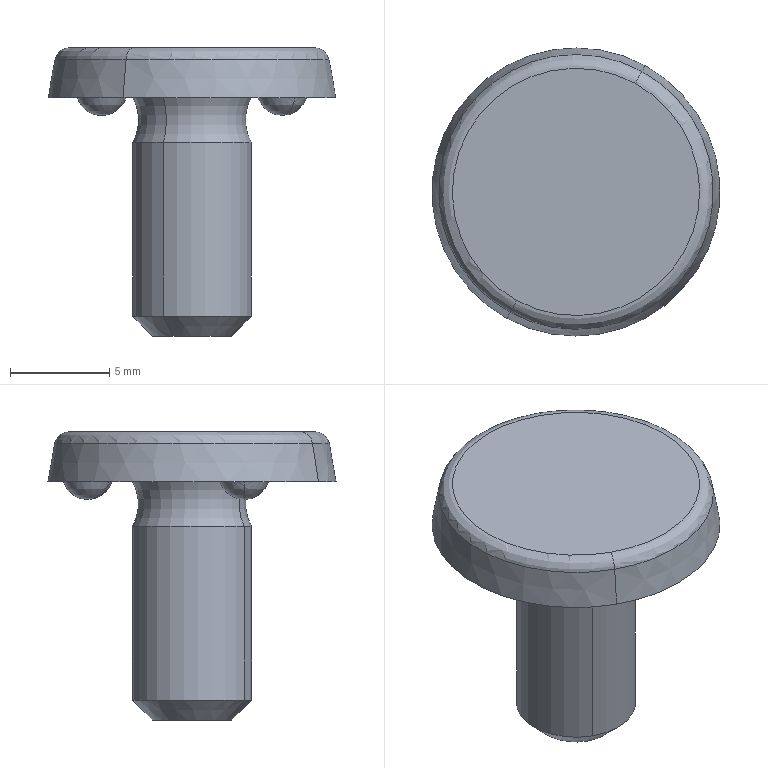Part | STEP file | Q1980612 | 1 solid | 19 faces | box 14.5 x 14.5 x 14.5 mm | volume 715.577 mm3 | sphere 6 | cone 4 | torus 4 | plane 3 | cylinder 2 | commonest cylinder face diameters 6 x2
STEP:
#1=CARTESIAN_POINT('',(4.547,-2.625,-0.9));
#2=VERTEX_POINT('',#1);
#3=CARTESIAN_POINT('',(5.19,-3.681,0.));
#4=VERTEX_POINT('',#3);
#5=CARTESIAN_POINT('',(4.547,-2.625,0.4));
#6=DIRECTION('',(0.854,0.5203,0.));
#7=AXIS2_PLACEMENT_3D('',#5,#6,$);
#8=CIRCLE('',#7,1.3);
#9=EDGE_CURVE('',#2,#4,#8,.F.);
#10=ORIENTED_EDGE('',*,*,#9,.F.);
#11=CARTESIAN_POINT('',(3.903,-1.569,0.));
#12=VERTEX_POINT('',#11);
#13=CARTESIAN_POINT('',(4.547,-2.625,0.4));
#14=DIRECTION('',(-0.854,-0.5203,0.));
#15=AXIS2_PLACEMENT_3D('',#13,#14,$);
#16=CIRCLE('',#15,1.3);
#17=EDGE_CURVE('',#2,#12,#16,.F.);
#18=ORIENTED_EDGE('',*,*,#17,.T.);
#19=CARTESIAN_POINT('',(5.19,-3.681,0.));
#20=CARTESIAN_POINT('',(5.46,-3.517,0.));
#21=CARTESIAN_POINT('',(5.678,-3.266,0.));
#22=CARTESIAN_POINT('',(5.805,-2.951,0.));
#23=CARTESIAN_POINT('',(5.832,-2.453,0.));
#24=CARTESIAN_POINT('',(5.639,-2.013,0.));
#25=CARTESIAN_POINT('',(5.551,-1.877,0.));
#26=CARTESIAN_POINT('',(5.238,-1.532,0.));
#27=CARTESIAN_POINT('',(4.79,-1.354,0.));
#28=CARTESIAN_POINT('',(4.468,-1.333,0.));
#29=CARTESIAN_POINT('',(4.161,-1.411,0.));
#30=CARTESIAN_POINT('',(3.903,-1.569,0.));
#31=B_SPLINE_CURVE_WITH_KNOTS('',5,(#19,#20,#21,#22,#23,#24,#25,#26,#27,#28,#29,#30),.UNSPECIFIED.,.F.,.U.,(6,3,3,6),(0.,2.294,3.444,5.637),.UNSPECIFIED.);
#32=EDGE_CURVE('',#4,#12,#31,.T.);
#33=ORIENTED_EDGE('',*,*,#32,.F.);
#34=EDGE_LOOP('',(#10,#18,#33));
#35=FACE_OUTER_BOUND('',#34,.T.);
#36=CARTESIAN_POINT('',(4.547,-2.625,0.4));
#37=DIRECTION('',(0.,0.,-1.));
#38=DIRECTION('',(0.5203,-0.854,0.));
#39=AXIS2_PLACEMENT_3D('',#36,#37,#38);
#40=SPHERICAL_SURFACE('',#39,1.3);
#41=ADVANCED_FACE('',(#35),#40,.T.);
#42=ORIENTED_EDGE('',*,*,#17,.F.);
#43=ORIENTED_EDGE('',*,*,#9,.T.);
#44=CARTESIAN_POINT('',(5.19,-3.681,0.));
#45=CARTESIAN_POINT('',(4.92,-3.846,0.));
#46=CARTESIAN_POINT('',(4.598,-3.924,0.));
#47=CARTESIAN_POINT('',(4.259,-3.893,0.));
#48=CARTESIAN_POINT('',(3.804,-3.689,0.));
#49=CARTESIAN_POINT('',(3.502,-3.315,0.));
#50=CARTESIAN_POINT('',(3.422,-3.175,0.));
#51=CARTESIAN_POINT('',(3.258,-2.738,0.));
#52=CARTESIAN_POINT('',(3.305,-2.258,0.));
#53=CARTESIAN_POINT('',(3.435,-1.962,0.));
#54=CARTESIAN_POINT('',(3.645,-1.726,0.));
#55=CARTESIAN_POINT('',(3.903,-1.569,0.));
#56=B_SPLINE_CURVE_WITH_KNOTS('',5,(#44,#45,#46,#47,#48,#49,#50,#51,#52,#53,#54,#55),.UNSPECIFIED.,.F.,.U.,(6,3,3,6),(0.,2.294,3.444,5.637),.UNSPECIFIED.);
#57=EDGE_CURVE('',#4,#12,#56,.T.);
#58=ORIENTED_EDGE('',*,*,#57,.T.);
#59=EDGE_LOOP('',(#42,#43,#58));
#60=FACE_OUTER_BOUND('',#59,.T.);
#61=ADVANCED_FACE('',(#60),#40,.T.);
#62=CARTESIAN_POINT('',(-3.476,-6.362,0.));
#63=VERTEX_POINT('',#62);
#64=CARTESIAN_POINT('',(3.476,6.362,0.));
#65=VERTEX_POINT('',#64);
#66=CARTESIAN_POINT('',(0.,0.,0.));
#67=DIRECTION('',(0.,0.,-1.));
#68=AXIS2_PLACEMENT_3D('',#66,#67,$);
#69=CIRCLE('',#68,7.25);
#70=EDGE_CURVE('',#63,#65,#69,.T.);
#71=ORIENTED_EDGE('',*,*,#70,.T.);
#72=CARTESIAN_POINT('',(0.,0.,0.));
#73=DIRECTION('',(0.,0.,-1.));
#74=AXIS2_PLACEMENT_3D('',#72,#73,$);
#75=CIRCLE('',#74,7.25);
#76=EDGE_CURVE('',#65,#63,#75,.T.);
#77=ORIENTED_EDGE('',*,*,#76,.T.);
#78=EDGE_LOOP('',(#71,#77));
#79=FACE_OUTER_BOUND('',#78,.T.);
#80=CARTESIAN_POINT('',(1.438,2.633,0.));
#81=VERTEX_POINT('',#80);
#82=CARTESIAN_POINT('',(-1.438,-2.633,0.));
#83=VERTEX_POINT('',#82);
#84=CARTESIAN_POINT('',(0.,0.,0.));
#85=DIRECTION('',(0.,0.,-1.));
#86=AXIS2_PLACEMENT_3D('',#84,#85,$);
#87=CIRCLE('',#86,3.);
#88=EDGE_CURVE('',#81,#83,#87,.T.);
#89=ORIENTED_EDGE('',*,*,#88,.F.);
#90=CARTESIAN_POINT('',(0.,0.,0.));
#91=DIRECTION('',(0.,0.,-1.));
#92=AXIS2_PLACEMENT_3D('',#90,#91,$);
#93=CIRCLE('',#92,3.);
#94=EDGE_CURVE('',#83,#81,#93,.T.);
#95=ORIENTED_EDGE('',*,*,#94,.F.);
#96=EDGE_LOOP('',(#89,#95));
#97=FACE_BOUND('',#96,.T.);
#98=CARTESIAN_POINT('',(-5.783,-2.654,0.));
#99=VERTEX_POINT('',#98);
#100=CARTESIAN_POINT('',(-3.31,-2.596,0.));
#101=VERTEX_POINT('',#100);
#102=CARTESIAN_POINT('',(-5.783,-2.654,0.));
#103=CARTESIAN_POINT('',(-5.787,-2.497,0.));
#104=CARTESIAN_POINT('',(-5.766,-2.338,0.));
#105=CARTESIAN_POINT('',(-5.719,-2.185,0.));
#106=CARTESIAN_POINT('',(-5.578,-1.897,0.));
#107=CARTESIAN_POINT('',(-5.355,-1.668,0.));
#108=CARTESIAN_POINT('',(-5.225,-1.572,0.));
#109=CARTESIAN_POINT('',(-4.939,-1.425,0.));
#110=CARTESIAN_POINT('',(-4.622,-1.375,0.));
#111=CARTESIAN_POINT('',(-4.46,-1.376,0.));
#112=CARTESIAN_POINT('',(-4.144,-1.429,0.));
#113=CARTESIAN_POINT('',(-3.859,-1.578,0.));
#114=CARTESIAN_POINT('',(-3.73,-1.675,0.));
#115=CARTESIAN_POINT('',(-3.519,-1.896,0.));
#116=CARTESIAN_POINT('',(-3.383,-2.17,0.));
#117=CARTESIAN_POINT('',(-3.338,-2.309,0.));
#118=CARTESIAN_POINT('',(-3.313,-2.452,0.));
#119=CARTESIAN_POINT('',(-3.31,-2.596,0.));
#120=B_SPLINE_CURVE_WITH_KNOTS('',5,(#102,#103,#104,#105,#106,#107,#108,#109,#110,#111,#112,#113,#114,#115,#116,#117,#118,#119),.UNSPECIFIED.,.F.,.U.,(6,3,3,3,3,6),(0.,1.143,2.294,3.444,4.595,5.637),.UNSPECIFIED.);
#121=EDGE_CURVE('',#99,#101,#120,.T.);
#122=ORIENTED_EDGE('',*,*,#121,.F.);
#123=CARTESIAN_POINT('',(-5.783,-2.654,0.));
#124=CARTESIAN_POINT('',(-5.78,-2.812,0.));
#125=CARTESIAN_POINT('',(-5.751,-2.969,0.));
#126=CARTESIAN_POINT('',(-5.697,-3.12,0.));
#127=CARTESIAN_POINT('',(-5.543,-3.4,0.));
#128=CARTESIAN_POINT('',(-5.309,-3.619,0.));
#129=CARTESIAN_POINT('',(-5.174,-3.709,0.));
#130=CARTESIAN_POINT('',(-4.882,-3.842,0.));
#131=CARTESIAN_POINT('',(-4.563,-3.877,0.));
#132=CARTESIAN_POINT('',(-4.402,-3.869,0.));
#133=CARTESIAN_POINT('',(-4.088,-3.801,0.));
#134=CARTESIAN_POINT('',(-3.811,-3.638,0.));
#135=CARTESIAN_POINT('',(-3.686,-3.535,0.));
#136=CARTESIAN_POINT('',(-3.485,-3.304,0.));
#137=CARTESIAN_POINT('',(-3.363,-3.024,0.));
#138=CARTESIAN_POINT('',(-3.324,-2.884,0.));
#139=CARTESIAN_POINT('',(-3.307,-2.74,0.));
#140=CARTESIAN_POINT('',(-3.31,-2.596,0.));
#141=B_SPLINE_CURVE_WITH_KNOTS('',5,(#123,#124,#125,#126,#127,#128,#129,#130,#131,#132,#133,#134,#135,#136,#137,#138,#139,#140),.UNSPECIFIED.,.F.,.U.,(6,3,3,3,3,6),(0.,1.143,2.294,3.444,4.595,5.637),.UNSPECIFIED.);
#142=EDGE_CURVE('',#99,#101,#141,.T.);
#143=ORIENTED_EDGE('',*,*,#142,.T.);
#144=EDGE_LOOP('',(#122,#143));
#145=FACE_BOUND('',#144,.T.);
#146=CARTESIAN_POINT('',(0.593,6.336,0.));
#147=VERTEX_POINT('',#146);
#148=CARTESIAN_POINT('',(-0.593,4.164,0.));
#149=VERTEX_POINT('',#148);
#150=CARTESIAN_POINT('',(0.593,6.336,0.));
#151=CARTESIAN_POINT('',(0.7313,6.26,0.));
#152=CARTESIAN_POINT('',(0.8576,6.162,0.));
#153=CARTESIAN_POINT('',(0.9672,6.045,0.));
#154=CARTESIAN_POINT('',(1.146,5.779,0.));
#155=CARTESIAN_POINT('',(1.233,5.471,0.));
#156=CARTESIAN_POINT('',(1.251,5.311,0.));
#157=CARTESIAN_POINT('',(1.235,4.99,0.));
#158=CARTESIAN_POINT('',(1.12,4.69,0.));
#159=CARTESIAN_POINT('',(1.039,4.551,0.));
#160=CARTESIAN_POINT('',(0.8345,4.303,0.));
#161=CARTESIAN_POINT('',(0.5629,4.131,0.));
#162=CARTESIAN_POINT('',(0.4143,4.068,0.));
#163=CARTESIAN_POINT('',(0.1169,3.995,0.));
#164=CARTESIAN_POINT('',(-0.188,4.015,0.));
#165=CARTESIAN_POINT('',(-0.3307,4.045,0.));
#166=CARTESIAN_POINT('',(-0.4669,4.096,0.));
#167=CARTESIAN_POINT('',(-0.593,4.164,0.));
#168=B_SPLINE_CURVE_WITH_KNOTS('',5,(#150,#151,#152,#153,#154,#155,#156,#157,#158,#159,#160,#161,#162,#163,#164,#165,#166,#167),.UNSPECIFIED.,.F.,.U.,(6,3,3,3,3,6),(0.,1.143,2.294,3.444,4.595,5.637),.UNSPECIFIED.);
#169=EDGE_CURVE('',#147,#149,#168,.T.);
#170=ORIENTED_EDGE('',*,*,#169,.F.);
#171=CARTESIAN_POINT('',(0.593,6.336,0.));
#172=CARTESIAN_POINT('',(0.4547,6.411,0.));
#173=CARTESIAN_POINT('',(0.3043,6.465,0.));
#174=CARTESIAN_POINT('',(0.1466,6.494,0.));
#175=CARTESIAN_POINT('',(-0.1735,6.5,0.));
#176=CARTESIAN_POINT('',(-0.4798,6.407,0.));
#177=CARTESIAN_POINT('',(-0.6246,6.335,0.));
#178=CARTESIAN_POINT('',(-0.8862,6.149,0.));
#179=CARTESIAN_POINT('',(-1.076,5.89,0.));
#180=CARTESIAN_POINT('',(-1.15,5.746,0.));
#181=CARTESIAN_POINT('',(-1.248,5.44,0.));
#182=CARTESIAN_POINT('',(-1.245,5.119,0.));
#183=CARTESIAN_POINT('',(-1.218,4.96,0.));
#184=CARTESIAN_POINT('',(-1.119,4.67,0.));
#185=CARTESIAN_POINT('',(-0.9379,4.424,0.));
#186=CARTESIAN_POINT('',(-0.8353,4.321,0.));
#187=CARTESIAN_POINT('',(-0.7192,4.233,0.));
#188=CARTESIAN_POINT('',(-0.593,4.164,0.));
#189=B_SPLINE_CURVE_WITH_KNOTS('',5,(#171,#172,#173,#174,#175,#176,#177,#178,#179,#180,#181,#182,#183,#184,#185,#186,#187,#188),.UNSPECIFIED.,.F.,.U.,(6,3,3,3,3,6),(0.,1.143,2.294,3.444,4.595,5.637),.UNSPECIFIED.);
#190=EDGE_CURVE('',#147,#149,#189,.T.);
#191=ORIENTED_EDGE('',*,*,#190,.T.);
#192=EDGE_LOOP('',(#170,#191));
#193=FACE_BOUND('',#192,.T.);
#194=ORIENTED_EDGE('',*,*,#57,.F.);
#195=ORIENTED_EDGE('',*,*,#32,.T.);
#196=EDGE_LOOP('',(#194,#195));
#197=FACE_BOUND('',#196,.T.);
#198=CARTESIAN_POINT('',(0.,3.,0.));
#199=DIRECTION('',(0.,0.,-1.));
#200=DIRECTION('',(1.,0.,0.));
#201=AXIS2_PLACEMENT_3D('',#198,#199,#200);
#202=PLANE('',#201);
#203=ADVANCED_FACE('',(#79,#97,#145,#193,#197),#202,.T.);
#204=ORIENTED_EDGE('',*,*,#70,.F.);
#205=CARTESIAN_POINT('',(-3.313,-6.065,1.922));
#206=VERTEX_POINT('',#205);
#207=CARTESIAN_POINT('',(-3.395,-6.214,0.9608));
#208=DIRECTION('',(-0.08325,-0.1524,-0.9848));
#209=VECTOR('',#208,1.);
#210=LINE('',#207,#209);
#211=EDGE_CURVE('',#63,#206,#210,.F.);
#212=ORIENTED_EDGE('',*,*,#211,.T.);
#213=CARTESIAN_POINT('',(3.313,6.065,1.922));
#214=VERTEX_POINT('',#213);
#215=CARTESIAN_POINT('',(0.,0.,1.922));
#216=DIRECTION('',(0.,0.,-1.));
#217=AXIS2_PLACEMENT_3D('',#215,#216,$);
#218=CIRCLE('',#217,6.911);
#219=EDGE_CURVE('',#206,#214,#218,.T.);
#220=ORIENTED_EDGE('',*,*,#219,.T.);
#221=CARTESIAN_POINT('',(3.395,6.214,0.9608));
#222=DIRECTION('',(0.08325,0.1524,-0.9848));
#223=VECTOR('',#222,1.);
#224=LINE('',#221,#223);
#225=EDGE_CURVE('',#65,#214,#224,.F.);
#226=ORIENTED_EDGE('',*,*,#225,.F.);
#227=EDGE_LOOP('',(#204,#212,#220,#226));
#228=FACE_OUTER_BOUND('',#227,.T.);
#229=CARTESIAN_POINT('',(0.,0.,1.922));
#230=DIRECTION('',(0.,0.,-1.));
#231=DIRECTION('',(0.4794,0.8776,0.));
#232=AXIS2_PLACEMENT_3D('',#229,#230,#231);
#233=CONICAL_SURFACE('',#232,6.911,0.1745);
#234=ADVANCED_FACE('',(#228),#233,.T.);
#235=ORIENTED_EDGE('',*,*,#76,.F.);
#236=ORIENTED_EDGE('',*,*,#225,.T.);
#237=CARTESIAN_POINT('',(0.,0.,1.922));
#238=DIRECTION('',(0.,0.,-1.));
#239=AXIS2_PLACEMENT_3D('',#237,#238,$);
#240=CIRCLE('',#239,6.911);
#241=EDGE_CURVE('',#214,#206,#240,.T.);
#242=ORIENTED_EDGE('',*,*,#241,.T.);
#243=ORIENTED_EDGE('',*,*,#211,.F.);
#244=EDGE_LOOP('',(#235,#236,#242,#243));
#245=FACE_OUTER_BOUND('',#244,.T.);
#246=ADVANCED_FACE('',(#245),#233,.T.);
#247=CARTESIAN_POINT('',(1.438,2.633,-2.25));
#248=VERTEX_POINT('',#247);
#249=CARTESIAN_POINT('',(-1.438,-2.633,-2.25));
#250=VERTEX_POINT('',#249);
#251=CARTESIAN_POINT('',(0.,0.,-2.25));
#252=DIRECTION('',(0.,0.,-1.));
#253=AXIS2_PLACEMENT_3D('',#251,#252,$);
#254=CIRCLE('',#253,3.);
#255=EDGE_CURVE('',#248,#250,#254,.T.);
#256=ORIENTED_EDGE('',*,*,#255,.F.);
#257=CARTESIAN_POINT('',(2.372,4.343,-1.125));
#258=DIRECTION('',(-0.8776,0.4794,0.));
#259=AXIS2_PLACEMENT_3D('',#257,#258,$);
#260=CIRCLE('',#259,2.25);
#261=EDGE_CURVE('',#248,#81,#260,.T.);
#262=ORIENTED_EDGE('',*,*,#261,.T.);
#263=ORIENTED_EDGE('',*,*,#88,.T.);
#264=CARTESIAN_POINT('',(-2.372,-4.343,-1.125));
#265=DIRECTION('',(0.8776,-0.4794,0.));
#266=AXIS2_PLACEMENT_3D('',#264,#265,$);
#267=CIRCLE('',#266,2.25);
#268=EDGE_CURVE('',#250,#83,#267,.T.);
#269=ORIENTED_EDGE('',*,*,#268,.F.);
#270=EDGE_LOOP('',(#256,#262,#263,#269));
#271=FACE_OUTER_BOUND('',#270,.T.);
#272=CARTESIAN_POINT('',(0.,0.,-1.125));
#273=DIRECTION('',(0.,0.,-1.));
#274=DIRECTION('',(0.4794,0.8776,0.));
#275=AXIS2_PLACEMENT_3D('',#272,#273,#274);
#276=TOROIDAL_SURFACE('',#275,4.949,2.25);
#277=ADVANCED_FACE('',(#271),#276,.F.);
#278=CARTESIAN_POINT('',(0.,0.,-2.25));
#279=DIRECTION('',(0.,0.,-1.));
#280=AXIS2_PLACEMENT_3D('',#278,#279,$);
#281=CIRCLE('',#280,3.);
#282=EDGE_CURVE('',#250,#248,#281,.T.);
#283=ORIENTED_EDGE('',*,*,#282,.F.);
#284=ORIENTED_EDGE('',*,*,#268,.T.);
#285=ORIENTED_EDGE('',*,*,#94,.T.);
#286=ORIENTED_EDGE('',*,*,#261,.F.);
#287=EDGE_LOOP('',(#283,#284,#285,#286));
#288=FACE_OUTER_BOUND('',#287,.T.);
#289=ADVANCED_FACE('',(#288),#276,.F.);
#290=CARTESIAN_POINT('',(-4.547,-2.625,-0.9));
#291=VERTEX_POINT('',#290);
#292=CARTESIAN_POINT('',(-4.547,-2.625,0.4));
#293=DIRECTION('',(-0.0236,0.9997,0.));
#294=AXIS2_PLACEMENT_3D('',#292,#293,$);
#295=CIRCLE('',#294,1.3);
#296=EDGE_CURVE('',#291,#101,#295,.F.);
#297=ORIENTED_EDGE('',*,*,#296,.F.);
#298=CARTESIAN_POINT('',(-4.547,-2.625,0.4));
#299=DIRECTION('',(0.0236,-0.9997,0.));
#300=AXIS2_PLACEMENT_3D('',#298,#299,$);
#301=CIRCLE('',#300,1.3);
#302=EDGE_CURVE('',#291,#99,#301,.F.);
#303=ORIENTED_EDGE('',*,*,#302,.T.);
#304=ORIENTED_EDGE('',*,*,#121,.T.);
#305=EDGE_LOOP('',(#297,#303,#304));
#306=FACE_OUTER_BOUND('',#305,.T.);
#307=CARTESIAN_POINT('',(-4.547,-2.625,0.4));
#308=DIRECTION('',(0.,0.,-1.));
#309=DIRECTION('',(-0.9997,-0.0236,0.));
#310=AXIS2_PLACEMENT_3D('',#307,#308,#309);
#311=SPHERICAL_SURFACE('',#310,1.3);
#312=ADVANCED_FACE('',(#306),#311,.T.);
#313=ORIENTED_EDGE('',*,*,#302,.F.);
#314=ORIENTED_EDGE('',*,*,#296,.T.);
#315=ORIENTED_EDGE('',*,*,#142,.F.);
#316=EDGE_LOOP('',(#313,#314,#315));
#317=FACE_OUTER_BOUND('',#316,.T.);
#318=ADVANCED_FACE('',(#317),#311,.T.);
#319=CARTESIAN_POINT('',(0.,5.25,-0.9));
#320=VERTEX_POINT('',#319);
#321=CARTESIAN_POINT('',(0.,5.25,0.4));
#322=DIRECTION('',(0.8776,-0.4794,0.));
#323=AXIS2_PLACEMENT_3D('',#321,#322,$);
#324=CIRCLE('',#323,1.3);
#325=EDGE_CURVE('',#320,#149,#324,.F.);
#326=ORIENTED_EDGE('',*,*,#325,.F.);
#327=CARTESIAN_POINT('',(0.,5.25,0.4));
#328=DIRECTION('',(-0.8776,0.4794,0.));
#329=AXIS2_PLACEMENT_3D('',#327,#328,$);
#330=CIRCLE('',#329,1.3);
#331=EDGE_CURVE('',#320,#147,#330,.F.);
#332=ORIENTED_EDGE('',*,*,#331,.T.);
#333=ORIENTED_EDGE('',*,*,#169,.T.);
#334=EDGE_LOOP('',(#326,#332,#333));
#335=FACE_OUTER_BOUND('',#334,.T.);
#336=CARTESIAN_POINT('',(0.,5.25,0.4));
#337=DIRECTION('',(0.,0.,-1.));
#338=DIRECTION('',(0.4794,0.8776,0.));
#339=AXIS2_PLACEMENT_3D('',#336,#337,#338);
#340=SPHERICAL_SURFACE('',#339,1.3);
#341=ADVANCED_FACE('',(#335),#340,.T.);
#342=ORIENTED_EDGE('',*,*,#331,.F.);
#343=ORIENTED_EDGE('',*,*,#325,.T.);
#344=ORIENTED_EDGE('',*,*,#190,.F.);
#345=EDGE_LOOP('',(#342,#343,#344));
#346=FACE_OUTER_BOUND('',#345,.T.);
#347=ADVANCED_FACE('',(#346),#340,.T.);
#348=ORIENTED_EDGE('',*,*,#219,.F.);
#349=CARTESIAN_POINT('',(-2.983,-5.46,2.5));
#350=VERTEX_POINT('',#349);
#351=CARTESIAN_POINT('',(-2.983,-5.46,1.8));
#352=DIRECTION('',(0.8776,-0.4794,0.));
#353=AXIS2_PLACEMENT_3D('',#351,#352,$);
#354=CIRCLE('',#353,0.7);
#355=EDGE_CURVE('',#206,#350,#354,.F.);
#356=ORIENTED_EDGE('',*,*,#355,.T.);
#357=CARTESIAN_POINT('',(2.983,5.46,2.5));
#358=VERTEX_POINT('',#357);
#359=CARTESIAN_POINT('',(0.,0.,2.5));
#360=DIRECTION('',(0.,0.,-1.));
#361=AXIS2_PLACEMENT_3D('',#359,#360,$);
#362=CIRCLE('',#361,6.222);
#363=EDGE_CURVE('',#350,#358,#362,.T.);
#364=ORIENTED_EDGE('',*,*,#363,.T.);
#365=CARTESIAN_POINT('',(2.983,5.46,1.8));
#366=DIRECTION('',(-0.8776,0.4794,0.));
#367=AXIS2_PLACEMENT_3D('',#365,#366,$);
#368=CIRCLE('',#367,0.7);
#369=EDGE_CURVE('',#214,#358,#368,.F.);
#370=ORIENTED_EDGE('',*,*,#369,.F.);
#371=EDGE_LOOP('',(#348,#356,#364,#370));
#372=FACE_OUTER_BOUND('',#371,.T.);
#373=CARTESIAN_POINT('',(0.,0.,1.8));
#374=DIRECTION('',(0.,0.,-1.));
#375=DIRECTION('',(0.4794,0.8776,0.));
#376=AXIS2_PLACEMENT_3D('',#373,#374,#375);
#377=TOROIDAL_SURFACE('',#376,6.222,0.7);
#378=ADVANCED_FACE('',(#372),#377,.T.);
#379=ORIENTED_EDGE('',*,*,#241,.F.);
#380=ORIENTED_EDGE('',*,*,#369,.T.);
#381=CARTESIAN_POINT('',(0.,0.,2.5));
#382=DIRECTION('',(0.,0.,-1.));
#383=AXIS2_PLACEMENT_3D('',#381,#382,$);
#384=CIRCLE('',#383,6.222);
#385=EDGE_CURVE('',#358,#350,#384,.T.);
#386=ORIENTED_EDGE('',*,*,#385,.T.);
#387=ORIENTED_EDGE('',*,*,#355,.F.);
#388=EDGE_LOOP('',(#379,#380,#386,#387));
#389=FACE_OUTER_BOUND('',#388,.T.);
#390=ADVANCED_FACE('',(#389),#377,.T.);
#391=CARTESIAN_POINT('',(1.438,2.633,-11.));
#392=VERTEX_POINT('',#391);
#393=CARTESIAN_POINT('',(-1.438,-2.633,-11.));
#394=VERTEX_POINT('',#393);
#395=CARTESIAN_POINT('',(0.,0.,-11.));
#396=DIRECTION('',(0.,0.,-1.));
#397=AXIS2_PLACEMENT_3D('',#395,#396,$);
#398=CIRCLE('',#397,3.);
#399=EDGE_CURVE('',#392,#394,#398,.T.);
#400=ORIENTED_EDGE('',*,*,#399,.F.);
#401=CARTESIAN_POINT('',(1.438,2.633,-6.625));
#402=DIRECTION('',(0.,0.,-1.));
#403=VECTOR('',#402,1.);
#404=LINE('',#401,#403);
#405=EDGE_CURVE('',#392,#248,#404,.F.);
#406=ORIENTED_EDGE('',*,*,#405,.T.);
#407=ORIENTED_EDGE('',*,*,#255,.T.);
#408=CARTESIAN_POINT('',(-1.438,-2.633,-6.625));
#409=DIRECTION('',(0.,0.,-1.));
#410=VECTOR('',#409,1.);
#411=LINE('',#408,#410);
#412=EDGE_CURVE('',#394,#250,#411,.F.);
#413=ORIENTED_EDGE('',*,*,#412,.F.);
#414=EDGE_LOOP('',(#400,#406,#407,#413));
#415=FACE_OUTER_BOUND('',#414,.T.);
#416=CARTESIAN_POINT('',(0.,0.,-4.75));
#417=DIRECTION('',(0.,0.,-1.));
#418=DIRECTION('',(0.4794,0.8776,0.));
#419=AXIS2_PLACEMENT_3D('',#416,#417,#418);
#420=CYLINDRICAL_SURFACE('',#419,3.);
#421=ADVANCED_FACE('',(#415),#420,.T.);
#422=CARTESIAN_POINT('',(0.,0.,-11.));
#423=DIRECTION('',(0.,0.,-1.));
#424=AXIS2_PLACEMENT_3D('',#422,#423,$);
#425=CIRCLE('',#424,3.);
#426=EDGE_CURVE('',#394,#392,#425,.T.);
#427=ORIENTED_EDGE('',*,*,#426,.F.);
#428=ORIENTED_EDGE('',*,*,#412,.T.);
#429=ORIENTED_EDGE('',*,*,#282,.T.);
#430=ORIENTED_EDGE('',*,*,#405,.F.);
#431=EDGE_LOOP('',(#427,#428,#429,#430));
#432=FACE_OUTER_BOUND('',#431,.T.);
#433=ADVANCED_FACE('',(#432),#420,.T.);
#434=ORIENTED_EDGE('',*,*,#385,.F.);
#435=ORIENTED_EDGE('',*,*,#363,.F.);
#436=EDGE_LOOP('',(#434,#435));
#437=FACE_OUTER_BOUND('',#436,.T.);
#438=CARTESIAN_POINT('',(0.,6.222,2.5));
#439=DIRECTION('',(0.,0.,-1.));
#440=DIRECTION('',(1.,0.,0.));
#441=AXIS2_PLACEMENT_3D('',#438,#439,#440);
#442=PLANE('',#441);
#443=ADVANCED_FACE('',(#437),#442,.F.);
#444=CARTESIAN_POINT('',(0.9589,1.755,-12.));
#445=VERTEX_POINT('',#444);
#446=CARTESIAN_POINT('',(-0.9589,-1.755,-12.));
#447=VERTEX_POINT('',#446);
#448=CARTESIAN_POINT('',(0.,0.,-12.));
#449=DIRECTION('',(0.,0.,1.));
#450=AXIS2_PLACEMENT_3D('',#448,#449,$);
#451=CIRCLE('',#450,2.);
#452=EDGE_CURVE('',#445,#447,#451,.F.);
#453=ORIENTED_EDGE('',*,*,#452,.F.);
#454=CARTESIAN_POINT('',(1.199,2.194,-11.5));
#455=DIRECTION('',(0.339,0.6205,0.7071));
#456=VECTOR('',#455,1.);
#457=LINE('',#454,#456);
#458=EDGE_CURVE('',#445,#392,#457,.T.);
#459=ORIENTED_EDGE('',*,*,#458,.T.);
#460=ORIENTED_EDGE('',*,*,#399,.T.);
#461=CARTESIAN_POINT('',(-1.199,-2.194,-11.5));
#462=DIRECTION('',(-0.339,-0.6205,0.7071));
#463=VECTOR('',#462,1.);
#464=LINE('',#461,#463);
#465=EDGE_CURVE('',#447,#394,#464,.T.);
#466=ORIENTED_EDGE('',*,*,#465,.F.);
#467=EDGE_LOOP('',(#453,#459,#460,#466));
#468=FACE_OUTER_BOUND('',#467,.T.);
#469=CARTESIAN_POINT('',(0.,0.,-12.));
#470=DIRECTION('',(0.,0.,1.));
#471=DIRECTION('',(0.4794,0.8776,0.));
#472=AXIS2_PLACEMENT_3D('',#469,#470,#471);
#473=CONICAL_SURFACE('',#472,2.,0.7854);
#474=ADVANCED_FACE('',(#468),#473,.T.);
#475=CARTESIAN_POINT('',(0.,0.,-12.));
#476=DIRECTION('',(0.,0.,1.));
#477=AXIS2_PLACEMENT_3D('',#475,#476,$);
#478=CIRCLE('',#477,2.);
#479=EDGE_CURVE('',#447,#445,#478,.F.);
#480=ORIENTED_EDGE('',*,*,#479,.F.);
#481=ORIENTED_EDGE('',*,*,#465,.T.);
#482=ORIENTED_EDGE('',*,*,#426,.T.);
#483=ORIENTED_EDGE('',*,*,#458,.F.);
#484=EDGE_LOOP('',(#480,#481,#482,#483));
#485=FACE_OUTER_BOUND('',#484,.T.);
#486=ADVANCED_FACE('',(#485),#473,.T.);
#487=ORIENTED_EDGE('',*,*,#452,.T.);
#488=ORIENTED_EDGE('',*,*,#479,.T.);
#489=EDGE_LOOP('',(#487,#488));
#490=FACE_OUTER_BOUND('',#489,.T.);
#491=CARTESIAN_POINT('',(0.,0.,-12.));
#492=DIRECTION('',(0.,0.,-1.));
#493=DIRECTION('',(1.,0.,0.));
#494=AXIS2_PLACEMENT_3D('',#491,#492,#493);
#495=PLANE('',#494);
#496=ADVANCED_FACE('',(#490),#495,.T.);
#497=CLOSED_SHELL('',(#41,#61,#203,#234,#246,#277,#289,#312,#318,#341,#347,#378,#390,#421,#433,#443,#474,#486,#496));
#498=MANIFOLD_SOLID_BREP('',#497);
#499=(LENGTH_UNIT()NAMED_UNIT(*)SI_UNIT(.MILLI.,.METRE.));
#500=UNCERTAINTY_MEASURE_WITH_UNIT(LENGTH_MEASURE(0.005),#499,'','');
#501=(NAMED_UNIT(*)PLANE_ANGLE_UNIT()SI_UNIT($,.RADIAN.));
#502=(NAMED_UNIT(*)SI_UNIT($,.STERADIAN.)SOLID_ANGLE_UNIT());
#503=(GEOMETRIC_REPRESENTATION_CONTEXT(3)GLOBAL_UNCERTAINTY_ASSIGNED_CONTEXT((#500))GLOBAL_UNIT_ASSIGNED_CONTEXT((#499,#501,#502))REPRESENTATION_CONTEXT('',''));
#504=ADVANCED_BREP_SHAPE_REPRESENTATION('',(#498),#503);